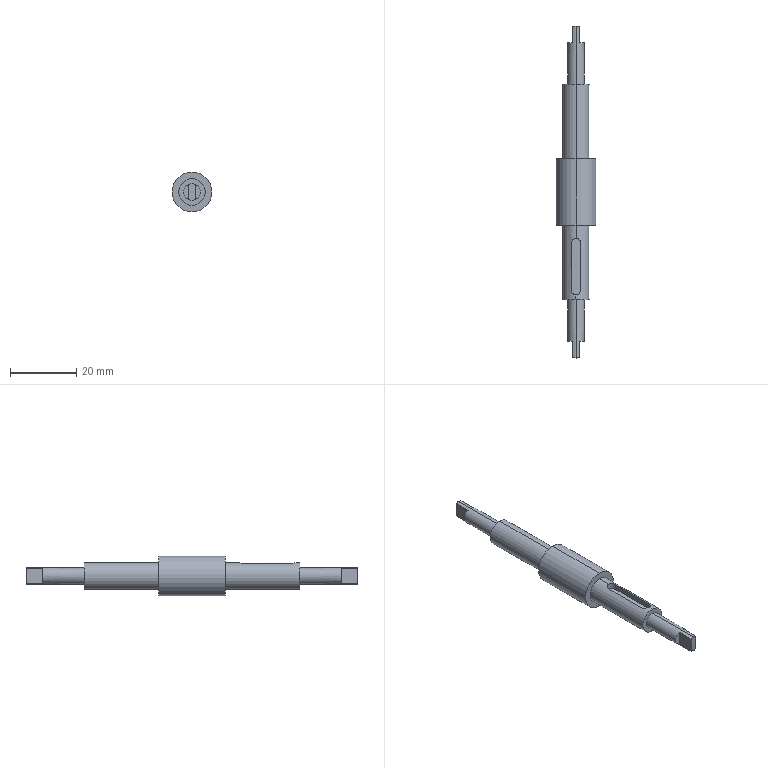Part | SolidWorks | features ICE 7, Extrusion 1 | 1 solid | 29 faces | box 12 x 100 x 12 mm | volume 5018 mm3 | plane 17 | cylinder 12 | commonest cylinder face diameters 5 x4 8 x4 3 x2 12 x2
STEP:
#1=CARTESIAN_POINT('',(0.,-50.,-2.5));
#2=VERTEX_POINT('',#1);
#3=CARTESIAN_POINT('',(1.,-50.,-2.291));
#4=VERTEX_POINT('',#3);
#5=CARTESIAN_POINT('',(0.,-50.,0.));
#6=DIRECTION('',(0.,-1.,0.));
#7=DIRECTION('',(0.,0.,-1.));
#8=AXIS2_PLACEMENT_3D('',#5,#6,#7);
#9=CIRCLE('',#8,2.5);
#10=EDGE_CURVE('',#2,#4,#9,.T.);
#11=ORIENTED_EDGE('',*,*,#10,.F.);
#12=CARTESIAN_POINT('',(0.,-32.5,-2.5));
#13=VERTEX_POINT('',#12);
#14=CARTESIAN_POINT('',(0.,-45.,-2.5));
#15=DIRECTION('',(0.,1.,0.));
#16=VECTOR('',#15,1000.);
#17=LINE('',#14,#16);
#18=EDGE_CURVE('',#2,#13,#17,.T.);
#19=ORIENTED_EDGE('',*,*,#18,.T.);
#20=CARTESIAN_POINT('',(0.,-32.5,2.5));
#21=VERTEX_POINT('',#20);
#22=CARTESIAN_POINT('',(0.,-32.5,0.));
#23=DIRECTION('',(0.,-1.,0.));
#24=DIRECTION('',(0.,0.,-1.));
#25=AXIS2_PLACEMENT_3D('',#22,#23,#24);
#26=CIRCLE('',#25,2.5);
#27=EDGE_CURVE('',#13,#21,#26,.T.);
#28=ORIENTED_EDGE('',*,*,#27,.T.);
#29=CARTESIAN_POINT('',(0.,-50.,2.5));
#30=VERTEX_POINT('',#29);
#31=CARTESIAN_POINT('',(0.,-45.,2.5));
#32=DIRECTION('',(0.,1.,0.));
#33=VECTOR('',#32,1000.);
#34=LINE('',#31,#33);
#35=EDGE_CURVE('',#30,#21,#34,.T.);
#36=ORIENTED_EDGE('',*,*,#35,.F.);
#37=CARTESIAN_POINT('',(1.,-50.,2.291));
#38=VERTEX_POINT('',#37);
#39=CARTESIAN_POINT('',(0.,-50.,0.));
#40=DIRECTION('',(0.,-1.,0.));
#41=DIRECTION('',(0.,0.,-1.));
#42=AXIS2_PLACEMENT_3D('',#39,#40,#41);
#43=CIRCLE('',#42,2.5);
#44=EDGE_CURVE('',#38,#30,#43,.T.);
#45=ORIENTED_EDGE('',*,*,#44,.F.);
#46=CARTESIAN_POINT('',(1.,-45.,2.291));
#47=VERTEX_POINT('',#46);
#48=CARTESIAN_POINT('',(1.,-50.,2.291));
#49=DIRECTION('',(0.,1.,0.));
#50=VECTOR('',#49,1000.);
#51=LINE('',#48,#50);
#52=EDGE_CURVE('',#38,#47,#51,.T.);
#53=ORIENTED_EDGE('',*,*,#52,.T.);
#54=CARTESIAN_POINT('',(1.,-45.,-2.291));
#55=VERTEX_POINT('',#54);
#56=CARTESIAN_POINT('',(0.,-45.,0.));
#57=DIRECTION('',(0.,-1.,0.));
#58=DIRECTION('',(0.,0.,-1.));
#59=AXIS2_PLACEMENT_3D('',#56,#57,#58);
#60=CIRCLE('',#59,2.5);
#61=EDGE_CURVE('',#55,#47,#60,.T.);
#62=ORIENTED_EDGE('',*,*,#61,.F.);
#63=CARTESIAN_POINT('',(1.,-50.,-2.291));
#64=DIRECTION('',(0.,1.,0.));
#65=VECTOR('',#64,1000.);
#66=LINE('',#63,#65);
#67=EDGE_CURVE('',#4,#55,#66,.T.);
#68=ORIENTED_EDGE('',*,*,#67,.F.);
#69=EDGE_LOOP('',(#11,#19,#28,#36,#45,#53,#62,#68));
#70=FACE_OUTER_BOUND('',#69,.T.);
#71=CARTESIAN_POINT('',(0.,-45.,0.));
#72=DIRECTION('',(0.,1.,0.));
#73=DIRECTION('',(0.,0.,1.));
#74=AXIS2_PLACEMENT_3D('',#71,#72,#73);
#75=CYLINDRICAL_SURFACE('',#74,2.5);
#76=ADVANCED_FACE('',(#70),#75,.T.);
#77=CARTESIAN_POINT('',(0.,-32.5,-4.));
#78=VERTEX_POINT('',#77);
#79=CARTESIAN_POINT('',(0.,-32.5,4.));
#80=VERTEX_POINT('',#79);
#81=CARTESIAN_POINT('',(0.,-32.5,0.));
#82=DIRECTION('',(0.,-1.,0.));
#83=DIRECTION('',(0.,0.,-1.));
#84=AXIS2_PLACEMENT_3D('',#81,#82,#83);
#85=CIRCLE('',#84,4.);
#86=EDGE_CURVE('',#78,#80,#85,.T.);
#87=ORIENTED_EDGE('',*,*,#86,.F.);
#88=CARTESIAN_POINT('',(0.,-10.,-4.));
#89=VERTEX_POINT('',#88);
#90=CARTESIAN_POINT('',(0.,-32.5,-4.));
#91=DIRECTION('',(0.,1.,0.));
#92=VECTOR('',#91,1000.);
#93=LINE('',#90,#92);
#94=EDGE_CURVE('',#78,#89,#93,.T.);
#95=ORIENTED_EDGE('',*,*,#94,.T.);
#96=CARTESIAN_POINT('',(0.,-10.,4.));
#97=VERTEX_POINT('',#96);
#98=CARTESIAN_POINT('',(0.,-10.,0.));
#99=DIRECTION('',(0.,-1.,0.));
#100=DIRECTION('',(0.,0.,-1.));
#101=AXIS2_PLACEMENT_3D('',#98,#99,#100);
#102=CIRCLE('',#101,4.);
#103=EDGE_CURVE('',#89,#97,#102,.T.);
#104=ORIENTED_EDGE('',*,*,#103,.T.);
#105=CARTESIAN_POINT('',(0.,-14.,4.));
#106=VERTEX_POINT('',#105);
#107=CARTESIAN_POINT('',(0.,-32.5,4.));
#108=DIRECTION('',(0.,1.,0.));
#109=VECTOR('',#108,1000.);
#110=LINE('',#107,#109);
#111=EDGE_CURVE('',#106,#97,#110,.T.);
#112=ORIENTED_EDGE('',*,*,#111,.F.);
#113=CARTESIAN_POINT('',(1.5,-15.5,3.708));
#114=VERTEX_POINT('',#113);
#115=CARTESIAN_POINT('',(0.,-14.,4.));
#116=CARTESIAN_POINT('',(0.0988,-14.,4.));
#117=CARTESIAN_POINT('',(0.1991,-14.01,3.996));
#118=CARTESIAN_POINT('',(0.3921,-14.049,3.982));
#119=CARTESIAN_POINT('',(0.486,-14.077,3.971));
#120=CARTESIAN_POINT('',(0.6687,-14.154,3.945));
#121=CARTESIAN_POINT('',(0.7547,-14.2,3.929));
#122=CARTESIAN_POINT('',(0.9162,-14.308,3.895));
#123=CARTESIAN_POINT('',(0.9924,-14.371,3.876));
#124=CARTESIAN_POINT('',(1.13,-14.509,3.838));
#125=CARTESIAN_POINT('',(1.191,-14.583,3.819));
#126=CARTESIAN_POINT('',(1.3,-14.745,3.783));
#127=CARTESIAN_POINT('',(1.347,-14.832,3.767));
#128=CARTESIAN_POINT('',(1.459,-15.102,3.725));
#129=CARTESIAN_POINT('',(1.5,-15.3,3.708));
#130=CARTESIAN_POINT('',(1.5,-15.5,3.708));
#131=B_SPLINE_CURVE_WITH_KNOTS('',3,(#115,#116,#117,#118,#119,#120,#121,#122,#123,#124,#125,#126,#127,#128,#129,#130),.UNSPECIFIED.,.F.,.F.,(4,2,2,2,2,2,2,4),(0.002367,0.002663,0.002958,0.003254,0.003549,0.003845,0.00414,0.004731),.UNSPECIFIED.);
#132=EDGE_CURVE('',#106,#114,#131,.T.);
#133=ORIENTED_EDGE('',*,*,#132,.T.);
#134=CARTESIAN_POINT('',(1.5,-29.5,3.708));
#135=VERTEX_POINT('',#134);
#136=CARTESIAN_POINT('',(1.5,-32.5,3.708));
#137=DIRECTION('',(0.,-1.,0.));
#138=VECTOR('',#137,1000.);
#139=LINE('',#136,#138);
#140=EDGE_CURVE('',#114,#135,#139,.T.);
#141=ORIENTED_EDGE('',*,*,#140,.T.);
#142=CARTESIAN_POINT('',(0.,-31.,4.));
#143=VERTEX_POINT('',#142);
#144=CARTESIAN_POINT('',(1.5,-29.5,3.708));
#145=CARTESIAN_POINT('',(1.5,-29.6,3.708));
#146=CARTESIAN_POINT('',(1.49,-29.698,3.712));
#147=CARTESIAN_POINT('',(1.451,-29.891,3.727));
#148=CARTESIAN_POINT('',(1.422,-29.987,3.739));
#149=CARTESIAN_POINT('',(1.309,-30.259,3.781));
#150=CARTESIAN_POINT('',(1.197,-30.424,3.819));
#151=CARTESIAN_POINT('',(0.9232,-30.698,3.895));
#152=CARTESIAN_POINT('',(0.7573,-30.809,3.932));
#153=CARTESIAN_POINT('',(0.4867,-30.922,3.971));
#154=CARTESIAN_POINT('',(0.3912,-30.951,3.982));
#155=CARTESIAN_POINT('',(0.197,-30.99,3.996));
#156=CARTESIAN_POINT('',(0.09895,-31.,4.));
#157=CARTESIAN_POINT('',(0.,-31.,4.));
#158=B_SPLINE_CURVE_WITH_KNOTS('',3,(#144,#145,#146,#147,#148,#149,#150,#151,#152,#153,#154,#155,#156,#157),.UNSPECIFIED.,.F.,.F.,(4,2,2,2,2,2,4),(0.,0.0002959,0.0005918,0.001184,0.001775,0.002071,0.002367),.UNSPECIFIED.);
#159=EDGE_CURVE('',#135,#143,#158,.T.);
#160=ORIENTED_EDGE('',*,*,#159,.T.);
#161=CARTESIAN_POINT('',(0.,-32.5,4.));
#162=DIRECTION('',(0.,1.,0.));
#163=VECTOR('',#162,1000.);
#164=LINE('',#161,#163);
#165=EDGE_CURVE('',#80,#143,#164,.T.);
#166=ORIENTED_EDGE('',*,*,#165,.F.);
#167=EDGE_LOOP('',(#87,#95,#104,#112,#133,#141,#160,#166));
#168=FACE_OUTER_BOUND('',#167,.T.);
#169=CARTESIAN_POINT('',(0.,-32.5,0.));
#170=DIRECTION('',(0.,1.,0.));
#171=DIRECTION('',(0.,0.,1.));
#172=AXIS2_PLACEMENT_3D('',#169,#170,#171);
#173=CYLINDRICAL_SURFACE('',#172,4.);
#174=ADVANCED_FACE('',(#168),#173,.T.);
#175=CARTESIAN_POINT('',(0.,50.,2.5));
#176=VERTEX_POINT('',#175);
#177=CARTESIAN_POINT('',(1.,50.,2.291));
#178=VERTEX_POINT('',#177);
#179=CARTESIAN_POINT('',(0.,50.,0.));
#180=DIRECTION('',(0.,1.,0.));
#181=DIRECTION('',(0.,0.,1.));
#182=AXIS2_PLACEMENT_3D('',#179,#180,#181);
#183=CIRCLE('',#182,2.5);
#184=EDGE_CURVE('',#176,#178,#183,.T.);
#185=ORIENTED_EDGE('',*,*,#184,.F.);
#186=CARTESIAN_POINT('',(0.,32.5,2.5));
#187=VERTEX_POINT('',#186);
#188=CARTESIAN_POINT('',(0.,45.,2.5));
#189=DIRECTION('',(0.,-1.,0.));
#190=VECTOR('',#189,1000.);
#191=LINE('',#188,#190);
#192=EDGE_CURVE('',#176,#187,#191,.T.);
#193=ORIENTED_EDGE('',*,*,#192,.T.);
#194=CARTESIAN_POINT('',(0.,32.5,-2.5));
#195=VERTEX_POINT('',#194);
#196=CARTESIAN_POINT('',(0.,32.5,0.));
#197=DIRECTION('',(0.,1.,0.));
#198=DIRECTION('',(0.,0.,1.));
#199=AXIS2_PLACEMENT_3D('',#196,#197,#198);
#200=CIRCLE('',#199,2.5);
#201=EDGE_CURVE('',#187,#195,#200,.T.);
#202=ORIENTED_EDGE('',*,*,#201,.T.);
#203=CARTESIAN_POINT('',(0.,50.,-2.5));
#204=VERTEX_POINT('',#203);
#205=CARTESIAN_POINT('',(0.,45.,-2.5));
#206=DIRECTION('',(0.,-1.,0.));
#207=VECTOR('',#206,1000.);
#208=LINE('',#205,#207);
#209=EDGE_CURVE('',#204,#195,#208,.T.);
#210=ORIENTED_EDGE('',*,*,#209,.F.);
#211=CARTESIAN_POINT('',(1.,50.,-2.291));
#212=VERTEX_POINT('',#211);
#213=CARTESIAN_POINT('',(0.,50.,0.));
#214=DIRECTION('',(0.,1.,0.));
#215=DIRECTION('',(0.,0.,1.));
#216=AXIS2_PLACEMENT_3D('',#213,#214,#215);
#217=CIRCLE('',#216,2.5);
#218=EDGE_CURVE('',#212,#204,#217,.T.);
#219=ORIENTED_EDGE('',*,*,#218,.F.);
#220=CARTESIAN_POINT('',(1.,45.,-2.291));
#221=VERTEX_POINT('',#220);
#222=CARTESIAN_POINT('',(1.,50.,-2.291));
#223=DIRECTION('',(0.,-1.,0.));
#224=VECTOR('',#223,1000.);
#225=LINE('',#222,#224);
#226=EDGE_CURVE('',#212,#221,#225,.T.);
#227=ORIENTED_EDGE('',*,*,#226,.T.);
#228=CARTESIAN_POINT('',(1.,45.,2.291));
#229=VERTEX_POINT('',#228);
#230=CARTESIAN_POINT('',(0.,45.,0.));
#231=DIRECTION('',(0.,1.,0.));
#232=DIRECTION('',(0.,0.,1.));
#233=AXIS2_PLACEMENT_3D('',#230,#231,#232);
#234=CIRCLE('',#233,2.5);
#235=EDGE_CURVE('',#229,#221,#234,.T.);
#236=ORIENTED_EDGE('',*,*,#235,.F.);
#237=CARTESIAN_POINT('',(1.,50.,2.291));
#238=DIRECTION('',(0.,-1.,0.));
#239=VECTOR('',#238,1000.);
#240=LINE('',#237,#239);
#241=EDGE_CURVE('',#178,#229,#240,.T.);
#242=ORIENTED_EDGE('',*,*,#241,.F.);
#243=EDGE_LOOP('',(#185,#193,#202,#210,#219,#227,#236,#242));
#244=FACE_OUTER_BOUND('',#243,.T.);
#245=CARTESIAN_POINT('',(0.,45.,0.));
#246=DIRECTION('',(0.,-1.,0.));
#247=DIRECTION('',(0.,0.,-1.));
#248=AXIS2_PLACEMENT_3D('',#245,#246,#247);
#249=CYLINDRICAL_SURFACE('',#248,2.5);
#250=ADVANCED_FACE('',(#244),#249,.T.);
#251=CARTESIAN_POINT('',(0.,32.5,4.));
#252=VERTEX_POINT('',#251);
#253=CARTESIAN_POINT('',(0.,32.5,-4.));
#254=VERTEX_POINT('',#253);
#255=CARTESIAN_POINT('',(0.,32.5,0.));
#256=DIRECTION('',(0.,1.,0.));
#257=DIRECTION('',(0.,0.,1.));
#258=AXIS2_PLACEMENT_3D('',#255,#256,#257);
#259=CIRCLE('',#258,4.);
#260=EDGE_CURVE('',#252,#254,#259,.T.);
#261=ORIENTED_EDGE('',*,*,#260,.F.);
#262=CARTESIAN_POINT('',(0.,10.,4.));
#263=VERTEX_POINT('',#262);
#264=CARTESIAN_POINT('',(0.,32.5,4.));
#265=DIRECTION('',(0.,-1.,0.));
#266=VECTOR('',#265,1000.);
#267=LINE('',#264,#266);
#268=EDGE_CURVE('',#252,#263,#267,.T.);
#269=ORIENTED_EDGE('',*,*,#268,.T.);
#270=CARTESIAN_POINT('',(0.,10.,-4.));
#271=VERTEX_POINT('',#270);
#272=CARTESIAN_POINT('',(0.,10.,0.));
#273=DIRECTION('',(0.,1.,0.));
#274=DIRECTION('',(0.,0.,1.));
#275=AXIS2_PLACEMENT_3D('',#272,#273,#274);
#276=CIRCLE('',#275,4.);
#277=EDGE_CURVE('',#263,#271,#276,.T.);
#278=ORIENTED_EDGE('',*,*,#277,.T.);
#279=CARTESIAN_POINT('',(0.,32.5,-4.));
#280=DIRECTION('',(0.,-1.,0.));
#281=VECTOR('',#280,1000.);
#282=LINE('',#279,#281);
#283=EDGE_CURVE('',#254,#271,#282,.T.);
#284=ORIENTED_EDGE('',*,*,#283,.F.);
#285=EDGE_LOOP('',(#261,#269,#278,#284));
#286=FACE_OUTER_BOUND('',#285,.T.);
#287=CARTESIAN_POINT('',(0.,32.5,0.));
#288=DIRECTION('',(0.,-1.,0.));
#289=DIRECTION('',(0.,0.,-1.));
#290=AXIS2_PLACEMENT_3D('',#287,#288,#289);
#291=CYLINDRICAL_SURFACE('',#290,4.);
#292=ADVANCED_FACE('',(#286),#291,.T.);
#293=CARTESIAN_POINT('',(0.,10.,6.));
#294=VERTEX_POINT('',#293);
#295=CARTESIAN_POINT('',(0.,10.,-6.));
#296=VERTEX_POINT('',#295);
#297=CARTESIAN_POINT('',(0.,10.,0.));
#298=DIRECTION('',(0.,1.,0.));
#299=DIRECTION('',(0.,0.,1.));
#300=AXIS2_PLACEMENT_3D('',#297,#298,#299);
#301=CIRCLE('',#300,6.);
#302=EDGE_CURVE('',#294,#296,#301,.T.);
#303=ORIENTED_EDGE('',*,*,#302,.F.);
#304=CARTESIAN_POINT('',(0.,-10.,6.));
#305=VERTEX_POINT('',#304);
#306=CARTESIAN_POINT('',(0.,10.,6.));
#307=DIRECTION('',(0.,-1.,0.));
#308=VECTOR('',#307,1000.);
#309=LINE('',#306,#308);
#310=EDGE_CURVE('',#294,#305,#309,.T.);
#311=ORIENTED_EDGE('',*,*,#310,.T.);
#312=CARTESIAN_POINT('',(0.,-10.,-6.));
#313=VERTEX_POINT('',#312);
#314=CARTESIAN_POINT('',(0.,-10.,0.));
#315=DIRECTION('',(0.,1.,0.));
#316=DIRECTION('',(0.,0.,1.));
#317=AXIS2_PLACEMENT_3D('',#314,#315,#316);
#318=CIRCLE('',#317,6.);
#319=EDGE_CURVE('',#305,#313,#318,.T.);
#320=ORIENTED_EDGE('',*,*,#319,.T.);
#321=CARTESIAN_POINT('',(0.,10.,-6.));
#322=DIRECTION('',(0.,-1.,0.));
#323=VECTOR('',#322,1000.);
#324=LINE('',#321,#323);
#325=EDGE_CURVE('',#296,#313,#324,.T.);
#326=ORIENTED_EDGE('',*,*,#325,.F.);
#327=EDGE_LOOP('',(#303,#311,#320,#326));
#328=FACE_OUTER_BOUND('',#327,.T.);
#329=CARTESIAN_POINT('',(0.,10.,0.));
#330=DIRECTION('',(0.,-1.,0.));
#331=DIRECTION('',(0.,0.,-1.));
#332=AXIS2_PLACEMENT_3D('',#329,#330,#331);
#333=CYLINDRICAL_SURFACE('',#332,6.);
#334=ADVANCED_FACE('',(#328),#333,.T.);
#335=CARTESIAN_POINT('',(1.,45.,-2.291));
#336=DIRECTION('',(0.,0.,-1.));
#337=VECTOR('',#336,1000.);
#338=LINE('',#335,#337);
#339=EDGE_CURVE('',#229,#221,#338,.T.);
#340=ORIENTED_EDGE('',*,*,#339,.F.);
#341=ORIENTED_EDGE('',*,*,#235,.T.);
#342=EDGE_LOOP('',(#340,#341));
#343=FACE_OUTER_BOUND('',#342,.T.);
#344=CARTESIAN_POINT('',(0.,45.,0.));
#345=DIRECTION('',(0.,1.,0.));
#346=DIRECTION('',(0.,0.,1.));
#347=AXIS2_PLACEMENT_3D('',#344,#345,#346);
#348=PLANE('',#347);
#349=ADVANCED_FACE('',(#343),#348,.T.);
#350=CARTESIAN_POINT('',(1.,-45.,2.291));
#351=DIRECTION('',(0.,0.,1.));
#352=VECTOR('',#351,1000.);
#353=LINE('',#350,#352);
#354=EDGE_CURVE('',#55,#47,#353,.T.);
#355=ORIENTED_EDGE('',*,*,#354,.F.);
#356=ORIENTED_EDGE('',*,*,#61,.T.);
#357=EDGE_LOOP('',(#355,#356));
#358=FACE_OUTER_BOUND('',#357,.T.);
#359=CARTESIAN_POINT('',(0.,-45.,0.));
#360=DIRECTION('',(0.,-1.,0.));
#361=DIRECTION('',(0.,0.,-1.));
#362=AXIS2_PLACEMENT_3D('',#359,#360,#361);
#363=PLANE('',#362);
#364=ADVANCED_FACE('',(#358),#363,.T.);
#365=ORIENTED_EDGE('',*,*,#310,.F.);
#366=CARTESIAN_POINT('',(0.,10.,0.));
#367=DIRECTION('',(0.,1.,0.));
#368=DIRECTION('',(0.,0.,1.));
#369=AXIS2_PLACEMENT_3D('',#366,#367,#368);
#370=CIRCLE('',#369,6.);
#371=EDGE_CURVE('',#296,#294,#370,.T.);
#372=ORIENTED_EDGE('',*,*,#371,.F.);
#373=ORIENTED_EDGE('',*,*,#325,.T.);
#374=CARTESIAN_POINT('',(0.,-10.,0.));
#375=DIRECTION('',(0.,1.,0.));
#376=DIRECTION('',(0.,0.,1.));
#377=AXIS2_PLACEMENT_3D('',#374,#375,#376);
#378=CIRCLE('',#377,6.);
#379=EDGE_CURVE('',#313,#305,#378,.T.);
#380=ORIENTED_EDGE('',*,*,#379,.T.);
#381=EDGE_LOOP('',(#365,#372,#373,#380));
#382=FACE_OUTER_BOUND('',#381,.T.);
#383=CARTESIAN_POINT('',(0.,10.,0.));
#384=DIRECTION('',(0.,-1.,0.));
#385=DIRECTION('',(0.,0.,-1.));
#386=AXIS2_PLACEMENT_3D('',#383,#384,#385);
#387=CYLINDRICAL_SURFACE('',#386,6.);
#388=ADVANCED_FACE('',(#382),#387,.T.);
#389=CARTESIAN_POINT('',(0.,10.,0.));
#390=DIRECTION('',(0.,1.,0.));
#391=DIRECTION('',(0.,0.,1.));
#392=AXIS2_PLACEMENT_3D('',#389,#390,#391);
#393=CIRCLE('',#392,4.);
#394=EDGE_CURVE('',#271,#263,#393,.T.);
#395=ORIENTED_EDGE('',*,*,#394,.F.);
#396=ORIENTED_EDGE('',*,*,#277,.F.);
#397=EDGE_LOOP('',(#395,#396));
#398=FACE_BOUND('',#397,.T.);
#399=ORIENTED_EDGE('',*,*,#371,.T.);
#400=ORIENTED_EDGE('',*,*,#302,.T.);
#401=EDGE_LOOP('',(#399,#400));
#402=FACE_OUTER_BOUND('',#401,.T.);
#403=CARTESIAN_POINT('',(0.,10.,0.));
#404=DIRECTION('',(0.,1.,0.));
#405=DIRECTION('',(0.,0.,1.));
#406=AXIS2_PLACEMENT_3D('',#403,#404,#405);
#407=PLANE('',#406);
#408=ADVANCED_FACE('',(#398,#402),#407,.T.);
#409=CARTESIAN_POINT('',(0.,-10.,0.));
#410=DIRECTION('',(0.,-1.,0.));
#411=DIRECTION('',(0.,0.,-1.));
#412=AXIS2_PLACEMENT_3D('',#409,#410,#411);
#413=CIRCLE('',#412,4.);
#414=EDGE_CURVE('',#97,#89,#413,.T.);
#415=ORIENTED_EDGE('',*,*,#414,.F.);
#416=ORIENTED_EDGE('',*,*,#103,.F.);
#417=EDGE_LOOP('',(#415,#416));
#418=FACE_BOUND('',#417,.T.);
#419=ORIENTED_EDGE('',*,*,#379,.F.);
#420=ORIENTED_EDGE('',*,*,#319,.F.);
#421=EDGE_LOOP('',(#419,#420));
#422=FACE_OUTER_BOUND('',#421,.T.);
#423=CARTESIAN_POINT('',(0.,-10.,0.));
#424=DIRECTION('',(0.,1.,0.));
#425=DIRECTION('',(0.,0.,1.));
#426=AXIS2_PLACEMENT_3D('',#423,#424,#425);
#427=PLANE('',#426);
#428=ADVANCED_FACE('',(#418,#422),#427,.F.);
#429=ORIENTED_EDGE('',*,*,#268,.F.);
#430=CARTESIAN_POINT('',(0.,32.5,0.));
#431=DIRECTION('',(0.,1.,0.));
#432=DIRECTION('',(0.,0.,1.));
#433=AXIS2_PLACEMENT_3D('',#430,#431,#432);
#434=CIRCLE('',#433,4.);
#435=EDGE_CURVE('',#254,#252,#434,.T.);
#436=ORIENTED_EDGE('',*,*,#435,.F.);
#437=ORIENTED_EDGE('',*,*,#283,.T.);
#438=ORIENTED_EDGE('',*,*,#394,.T.);
#439=EDGE_LOOP('',(#429,#436,#437,#438));
#440=FACE_OUTER_BOUND('',#439,.T.);
#441=CARTESIAN_POINT('',(0.,32.5,0.));
#442=DIRECTION('',(0.,-1.,0.));
#443=DIRECTION('',(0.,0.,-1.));
#444=AXIS2_PLACEMENT_3D('',#441,#442,#443);
#445=CYLINDRICAL_SURFACE('',#444,4.);
#446=ADVANCED_FACE('',(#440),#445,.T.);
#447=CARTESIAN_POINT('',(0.,32.5,0.));
#448=DIRECTION('',(0.,1.,0.));
#449=DIRECTION('',(0.,0.,1.));
#450=AXIS2_PLACEMENT_3D('',#447,#448,#449);
#451=CIRCLE('',#450,2.5);
#452=EDGE_CURVE('',#195,#187,#451,.T.);
#453=ORIENTED_EDGE('',*,*,#452,.F.);
#454=ORIENTED_EDGE('',*,*,#201,.F.);
#455=EDGE_LOOP('',(#453,#454));
#456=FACE_BOUND('',#455,.T.);
#457=ORIENTED_EDGE('',*,*,#435,.T.);
#458=ORIENTED_EDGE('',*,*,#260,.T.);
#459=EDGE_LOOP('',(#457,#458));
#460=FACE_OUTER_BOUND('',#459,.T.);
#461=CARTESIAN_POINT('',(0.,32.5,0.));
#462=DIRECTION('',(0.,1.,0.));
#463=DIRECTION('',(0.,0.,1.));
#464=AXIS2_PLACEMENT_3D('',#461,#462,#463);
#465=PLANE('',#464);
#466=ADVANCED_FACE('',(#456,#460),#465,.T.);
#467=ORIENTED_EDGE('',*,*,#192,.F.);
#468=CARTESIAN_POINT('',(-1.,50.,2.291));
#469=VERTEX_POINT('',#468);
#470=CARTESIAN_POINT('',(0.,50.,0.));
#471=DIRECTION('',(0.,1.,0.));
#472=DIRECTION('',(0.,0.,1.));
#473=AXIS2_PLACEMENT_3D('',#470,#471,#472);
#474=CIRCLE('',#473,2.5);
#475=EDGE_CURVE('',#469,#176,#474,.T.);
#476=ORIENTED_EDGE('',*,*,#475,.F.);
#477=CARTESIAN_POINT('',(-1.,45.,2.291));
#478=VERTEX_POINT('',#477);
#479=CARTESIAN_POINT('',(-1.,50.,2.291));
#480=DIRECTION('',(0.,-1.,0.));
#481=VECTOR('',#480,1000.);
#482=LINE('',#479,#481);
#483=EDGE_CURVE('',#469,#478,#482,.T.);
#484=ORIENTED_EDGE('',*,*,#483,.T.);
#485=CARTESIAN_POINT('',(-1.,45.,-2.291));
#486=VERTEX_POINT('',#485);
#487=CARTESIAN_POINT('',(0.,45.,0.));
#488=DIRECTION('',(0.,1.,0.));
#489=DIRECTION('',(0.,0.,1.));
#490=AXIS2_PLACEMENT_3D('',#487,#488,#489);
#491=CIRCLE('',#490,2.5);
#492=EDGE_CURVE('',#486,#478,#491,.T.);
#493=ORIENTED_EDGE('',*,*,#492,.F.);
#494=CARTESIAN_POINT('',(-1.,50.,-2.291));
#495=VERTEX_POINT('',#494);
#496=CARTESIAN_POINT('',(-1.,50.,-2.291));
#497=DIRECTION('',(0.,-1.,0.));
#498=VECTOR('',#497,1000.);
#499=LINE('',#496,#498);
#500=EDGE_CURVE('',#495,#486,#499,.T.);
#501=ORIENTED_EDGE('',*,*,#500,.F.);
#502=CARTESIAN_POINT('',(0.,50.,0.));
#503=DIRECTION('',(0.,1.,0.));
#504=DIRECTION('',(0.,0.,1.));
#505=AXIS2_PLACEMENT_3D('',#502,#503,#504);
#506=CIRCLE('',#505,2.5);
#507=EDGE_CURVE('',#204,#495,#506,.T.);
#508=ORIENTED_EDGE('',*,*,#507,.F.);
#509=ORIENTED_EDGE('',*,*,#209,.T.);
#510=ORIENTED_EDGE('',*,*,#452,.T.);
#511=EDGE_LOOP('',(#467,#476,#484,#493,#501,#508,#509,#510));
#512=FACE_OUTER_BOUND('',#511,.T.);
#513=CARTESIAN_POINT('',(0.,45.,0.));
#514=DIRECTION('',(0.,-1.,0.));
#515=DIRECTION('',(0.,0.,-1.));
#516=AXIS2_PLACEMENT_3D('',#513,#514,#515);
#517=CYLINDRICAL_SURFACE('',#516,2.5);
#518=ADVANCED_FACE('',(#512),#517,.T.);
#519=CARTESIAN_POINT('',(-1.,45.,-2.291));
#520=DIRECTION('',(0.,0.,1.));
#521=VECTOR('',#520,1000.);
#522=LINE('',#519,#521);
#523=EDGE_CURVE('',#486,#478,#522,.T.);
#524=ORIENTED_EDGE('',*,*,#523,.F.);
#525=ORIENTED_EDGE('',*,*,#492,.T.);
#526=EDGE_LOOP('',(#524,#525));
#527=FACE_OUTER_BOUND('',#526,.T.);
#528=CARTESIAN_POINT('',(0.,45.,0.));
#529=DIRECTION('',(0.,1.,0.));
#530=DIRECTION('',(0.,0.,1.));
#531=AXIS2_PLACEMENT_3D('',#528,#529,#530);
#532=PLANE('',#531);
#533=ADVANCED_FACE('',(#527),#532,.T.);
#534=ORIENTED_EDGE('',*,*,#94,.F.);
#535=CARTESIAN_POINT('',(0.,-32.5,0.));
#536=DIRECTION('',(0.,-1.,0.));
#537=DIRECTION('',(0.,0.,-1.));
#538=AXIS2_PLACEMENT_3D('',#535,#536,#537);
#539=CIRCLE('',#538,4.);
#540=EDGE_CURVE('',#80,#78,#539,.T.);
#541=ORIENTED_EDGE('',*,*,#540,.F.);
#542=ORIENTED_EDGE('',*,*,#165,.T.);
#543=CARTESIAN_POINT('',(-1.5,-29.5,3.708));
#544=VERTEX_POINT('',#543);
#545=CARTESIAN_POINT('',(0.,-31.,4.));
#546=CARTESIAN_POINT('',(-0.0988,-31.,4.));
#547=CARTESIAN_POINT('',(-0.1991,-30.99,3.996));
#548=CARTESIAN_POINT('',(-0.3921,-30.951,3.982));
#549=CARTESIAN_POINT('',(-0.486,-30.923,3.971));
#550=CARTESIAN_POINT('',(-0.6687,-30.846,3.945));
#551=CARTESIAN_POINT('',(-0.7547,-30.8,3.929));
#552=CARTESIAN_POINT('',(-0.9162,-30.692,3.895));
#553=CARTESIAN_POINT('',(-0.9924,-30.629,3.876));
#554=CARTESIAN_POINT('',(-1.13,-30.491,3.838));
#555=CARTESIAN_POINT('',(-1.191,-30.417,3.819));
#556=CARTESIAN_POINT('',(-1.3,-30.255,3.783));
#557=CARTESIAN_POINT('',(-1.347,-30.168,3.767));
#558=CARTESIAN_POINT('',(-1.459,-29.898,3.725));
#559=CARTESIAN_POINT('',(-1.5,-29.7,3.708));
#560=CARTESIAN_POINT('',(-1.5,-29.5,3.708));
#561=B_SPLINE_CURVE_WITH_KNOTS('',3,(#545,#546,#547,#548,#549,#550,#551,#552,#553,#554,#555,#556,#557,#558,#559,#560),.UNSPECIFIED.,.F.,.F.,(4,2,2,2,2,2,2,4),(0.002367,0.002663,0.002958,0.003254,0.003549,0.003845,0.00414,0.004731),.UNSPECIFIED.);
#562=EDGE_CURVE('',#143,#544,#561,.T.);
#563=ORIENTED_EDGE('',*,*,#562,.T.);
#564=CARTESIAN_POINT('',(-1.5,-15.5,3.708));
#565=VERTEX_POINT('',#564);
#566=CARTESIAN_POINT('',(-1.5,-32.5,3.708));
#567=DIRECTION('',(0.,1.,0.));
#568=VECTOR('',#567,1000.);
#569=LINE('',#566,#568);
#570=EDGE_CURVE('',#544,#565,#569,.T.);
#571=ORIENTED_EDGE('',*,*,#570,.T.);
#572=CARTESIAN_POINT('',(-1.5,-15.5,3.708));
#573=CARTESIAN_POINT('',(-1.5,-15.4,3.708));
#574=CARTESIAN_POINT('',(-1.49,-15.302,3.712));
#575=CARTESIAN_POINT('',(-1.451,-15.109,3.727));
#576=CARTESIAN_POINT('',(-1.422,-15.013,3.739));
#577=CARTESIAN_POINT('',(-1.309,-14.741,3.781));
#578=CARTESIAN_POINT('',(-1.197,-14.576,3.819));
#579=CARTESIAN_POINT('',(-0.9232,-14.302,3.895));
#580=CARTESIAN_POINT('',(-0.7573,-14.191,3.932));
#581=CARTESIAN_POINT('',(-0.4867,-14.078,3.971));
#582=CARTESIAN_POINT('',(-0.3912,-14.049,3.982));
#583=CARTESIAN_POINT('',(-0.197,-14.01,3.996));
#584=CARTESIAN_POINT('',(-0.09895,-14.,4.));
#585=CARTESIAN_POINT('',(0.,-14.,4.));
#586=B_SPLINE_CURVE_WITH_KNOTS('',3,(#572,#573,#574,#575,#576,#577,#578,#579,#580,#581,#582,#583,#584,#585),.UNSPECIFIED.,.F.,.F.,(4,2,2,2,2,2,4),(0.,0.0002959,0.0005918,0.001184,0.001775,0.002071,0.002367),.UNSPECIFIED.);
#587=EDGE_CURVE('',#565,#106,#586,.T.);
#588=ORIENTED_EDGE('',*,*,#587,.T.);
#589=ORIENTED_EDGE('',*,*,#111,.T.);
#590=ORIENTED_EDGE('',*,*,#414,.T.);
#591=EDGE_LOOP('',(#534,#541,#542,#563,#571,#588,#589,#590));
#592=FACE_OUTER_BOUND('',#591,.T.);
#593=CARTESIAN_POINT('',(0.,-32.5,0.));
#594=DIRECTION('',(0.,1.,0.));
#595=DIRECTION('',(0.,0.,1.));
#596=AXIS2_PLACEMENT_3D('',#593,#594,#595);
#597=CYLINDRICAL_SURFACE('',#596,4.);
#598=ADVANCED_FACE('',(#592),#597,.T.);
#599=CARTESIAN_POINT('',(0.,-32.5,0.));
#600=DIRECTION('',(0.,-1.,0.));
#601=DIRECTION('',(0.,0.,-1.));
#602=AXIS2_PLACEMENT_3D('',#599,#600,#601);
#603=CIRCLE('',#602,2.5);
#604=EDGE_CURVE('',#21,#13,#603,.T.);
#605=ORIENTED_EDGE('',*,*,#604,.F.);
#606=ORIENTED_EDGE('',*,*,#27,.F.);
#607=EDGE_LOOP('',(#605,#606));
#608=FACE_BOUND('',#607,.T.);
#609=ORIENTED_EDGE('',*,*,#540,.T.);
#610=ORIENTED_EDGE('',*,*,#86,.T.);
#611=EDGE_LOOP('',(#609,#610));
#612=FACE_OUTER_BOUND('',#611,.T.);
#613=CARTESIAN_POINT('',(0.,-32.5,0.));
#614=DIRECTION('',(0.,-1.,0.));
#615=DIRECTION('',(0.,0.,-1.));
#616=AXIS2_PLACEMENT_3D('',#613,#614,#615);
#617=PLANE('',#616);
#618=ADVANCED_FACE('',(#608,#612),#617,.T.);
#619=ORIENTED_EDGE('',*,*,#18,.F.);
#620=CARTESIAN_POINT('',(-1.,-50.,-2.291));
#621=VERTEX_POINT('',#620);
#622=CARTESIAN_POINT('',(0.,-50.,0.));
#623=DIRECTION('',(0.,-1.,0.));
#624=DIRECTION('',(0.,0.,-1.));
#625=AXIS2_PLACEMENT_3D('',#622,#623,#624);
#626=CIRCLE('',#625,2.5);
#627=EDGE_CURVE('',#621,#2,#626,.T.);
#628=ORIENTED_EDGE('',*,*,#627,.F.);
#629=CARTESIAN_POINT('',(-1.,-45.,-2.291));
#630=VERTEX_POINT('',#629);
#631=CARTESIAN_POINT('',(-1.,-50.,-2.291));
#632=DIRECTION('',(0.,1.,0.));
#633=VECTOR('',#632,1000.);
#634=LINE('',#631,#633);
#635=EDGE_CURVE('',#621,#630,#634,.T.);
#636=ORIENTED_EDGE('',*,*,#635,.T.);
#637=CARTESIAN_POINT('',(-1.,-45.,2.291));
#638=VERTEX_POINT('',#637);
#639=CARTESIAN_POINT('',(0.,-45.,0.));
#640=DIRECTION('',(0.,-1.,0.));
#641=DIRECTION('',(0.,0.,-1.));
#642=AXIS2_PLACEMENT_3D('',#639,#640,#641);
#643=CIRCLE('',#642,2.5);
#644=EDGE_CURVE('',#638,#630,#643,.T.);
#645=ORIENTED_EDGE('',*,*,#644,.F.);
#646=CARTESIAN_POINT('',(-1.,-50.,2.291));
#647=VERTEX_POINT('',#646);
#648=CARTESIAN_POINT('',(-1.,-50.,2.291));
#649=DIRECTION('',(0.,1.,0.));
#650=VECTOR('',#649,1000.);
#651=LINE('',#648,#650);
#652=EDGE_CURVE('',#647,#638,#651,.T.);
#653=ORIENTED_EDGE('',*,*,#652,.F.);
#654=CARTESIAN_POINT('',(0.,-50.,0.));
#655=DIRECTION('',(0.,-1.,0.));
#656=DIRECTION('',(0.,0.,-1.));
#657=AXIS2_PLACEMENT_3D('',#654,#655,#656);
#658=CIRCLE('',#657,2.5);
#659=EDGE_CURVE('',#30,#647,#658,.T.);
#660=ORIENTED_EDGE('',*,*,#659,.F.);
#661=ORIENTED_EDGE('',*,*,#35,.T.);
#662=ORIENTED_EDGE('',*,*,#604,.T.);
#663=EDGE_LOOP('',(#619,#628,#636,#645,#653,#660,#661,#662));
#664=FACE_OUTER_BOUND('',#663,.T.);
#665=CARTESIAN_POINT('',(0.,-45.,0.));
#666=DIRECTION('',(0.,1.,0.));
#667=DIRECTION('',(0.,0.,1.));
#668=AXIS2_PLACEMENT_3D('',#665,#666,#667);
#669=CYLINDRICAL_SURFACE('',#668,2.5);
#670=ADVANCED_FACE('',(#664),#669,.T.);
#671=CARTESIAN_POINT('',(-1.,-45.,2.291));
#672=DIRECTION('',(0.,0.,-1.));
#673=VECTOR('',#672,1000.);
#674=LINE('',#671,#673);
#675=EDGE_CURVE('',#638,#630,#674,.T.);
#676=ORIENTED_EDGE('',*,*,#675,.F.);
#677=ORIENTED_EDGE('',*,*,#644,.T.);
#678=EDGE_LOOP('',(#676,#677));
#679=FACE_OUTER_BOUND('',#678,.T.);
#680=CARTESIAN_POINT('',(0.,-45.,0.));
#681=DIRECTION('',(0.,-1.,0.));
#682=DIRECTION('',(0.,0.,-1.));
#683=AXIS2_PLACEMENT_3D('',#680,#681,#682);
#684=PLANE('',#683);
#685=ADVANCED_FACE('',(#679),#684,.T.);
#686=ORIENTED_EDGE('',*,*,#675,.T.);
#687=ORIENTED_EDGE('',*,*,#635,.F.);
#688=CARTESIAN_POINT('',(-1.,-50.,2.291));
#689=DIRECTION('',(0.,0.,-1.));
#690=VECTOR('',#689,1000.);
#691=LINE('',#688,#690);
#692=EDGE_CURVE('',#647,#621,#691,.T.);
#693=ORIENTED_EDGE('',*,*,#692,.F.);
#694=ORIENTED_EDGE('',*,*,#652,.T.);
#695=EDGE_LOOP('',(#686,#687,#693,#694));
#696=FACE_OUTER_BOUND('',#695,.T.);
#697=CARTESIAN_POINT('',(-1.,-50.,2.291));
#698=DIRECTION('',(1.,0.,0.));
#699=DIRECTION('',(0.,0.,-1.));
#700=AXIS2_PLACEMENT_3D('',#697,#698,#699);
#701=PLANE('',#700);
#702=ADVANCED_FACE('',(#696),#701,.F.);
#703=ORIENTED_EDGE('',*,*,#354,.T.);
#704=ORIENTED_EDGE('',*,*,#52,.F.);
#705=CARTESIAN_POINT('',(1.,-50.,2.291));
#706=DIRECTION('',(0.,0.,1.));
#707=VECTOR('',#706,1000.);
#708=LINE('',#705,#707);
#709=EDGE_CURVE('',#4,#38,#708,.T.);
#710=ORIENTED_EDGE('',*,*,#709,.F.);
#711=ORIENTED_EDGE('',*,*,#67,.T.);
#712=EDGE_LOOP('',(#703,#704,#710,#711));
#713=FACE_OUTER_BOUND('',#712,.T.);
#714=CARTESIAN_POINT('',(1.,-50.,2.291));
#715=DIRECTION('',(-1.,0.,0.));
#716=DIRECTION('',(0.,0.,1.));
#717=AXIS2_PLACEMENT_3D('',#714,#715,#716);
#718=PLANE('',#717);
#719=ADVANCED_FACE('',(#713),#718,.F.);
#720=ORIENTED_EDGE('',*,*,#44,.T.);
#721=ORIENTED_EDGE('',*,*,#659,.T.);
#722=ORIENTED_EDGE('',*,*,#692,.T.);
#723=ORIENTED_EDGE('',*,*,#627,.T.);
#724=ORIENTED_EDGE('',*,*,#10,.T.);
#725=ORIENTED_EDGE('',*,*,#709,.T.);
#726=EDGE_LOOP('',(#720,#721,#722,#723,#724,#725));
#727=FACE_OUTER_BOUND('',#726,.T.);
#728=CARTESIAN_POINT('',(0.,-50.,0.));
#729=DIRECTION('',(0.,-1.,0.));
#730=DIRECTION('',(0.,0.,-1.));
#731=AXIS2_PLACEMENT_3D('',#728,#729,#730);
#732=PLANE('',#731);
#733=ADVANCED_FACE('',(#727),#732,.T.);
#734=ORIENTED_EDGE('',*,*,#523,.T.);
#735=ORIENTED_EDGE('',*,*,#483,.F.);
#736=CARTESIAN_POINT('',(-1.,50.,-2.291));
#737=DIRECTION('',(0.,0.,1.));
#738=VECTOR('',#737,1000.);
#739=LINE('',#736,#738);
#740=EDGE_CURVE('',#495,#469,#739,.T.);
#741=ORIENTED_EDGE('',*,*,#740,.F.);
#742=ORIENTED_EDGE('',*,*,#500,.T.);
#743=EDGE_LOOP('',(#734,#735,#741,#742));
#744=FACE_OUTER_BOUND('',#743,.T.);
#745=CARTESIAN_POINT('',(-1.,50.,-2.291));
#746=DIRECTION('',(1.,0.,0.));
#747=DIRECTION('',(0.,0.,-1.));
#748=AXIS2_PLACEMENT_3D('',#745,#746,#747);
#749=PLANE('',#748);
#750=ADVANCED_FACE('',(#744),#749,.F.);
#751=ORIENTED_EDGE('',*,*,#339,.T.);
#752=ORIENTED_EDGE('',*,*,#226,.F.);
#753=CARTESIAN_POINT('',(1.,50.,-2.291));
#754=DIRECTION('',(0.,0.,-1.));
#755=VECTOR('',#754,1000.);
#756=LINE('',#753,#755);
#757=EDGE_CURVE('',#178,#212,#756,.T.);
#758=ORIENTED_EDGE('',*,*,#757,.F.);
#759=ORIENTED_EDGE('',*,*,#241,.T.);
#760=EDGE_LOOP('',(#751,#752,#758,#759));
#761=FACE_OUTER_BOUND('',#760,.T.);
#762=CARTESIAN_POINT('',(1.,50.,-2.291));
#763=DIRECTION('',(-1.,0.,0.));
#764=DIRECTION('',(0.,0.,1.));
#765=AXIS2_PLACEMENT_3D('',#762,#763,#764);
#766=PLANE('',#765);
#767=ADVANCED_FACE('',(#761),#766,.F.);
#768=ORIENTED_EDGE('',*,*,#218,.T.);
#769=ORIENTED_EDGE('',*,*,#507,.T.);
#770=ORIENTED_EDGE('',*,*,#740,.T.);
#771=ORIENTED_EDGE('',*,*,#475,.T.);
#772=ORIENTED_EDGE('',*,*,#184,.T.);
#773=ORIENTED_EDGE('',*,*,#757,.T.);
#774=EDGE_LOOP('',(#768,#769,#770,#771,#772,#773));
#775=FACE_OUTER_BOUND('',#774,.T.);
#776=CARTESIAN_POINT('',(0.,50.,0.));
#777=DIRECTION('',(0.,1.,0.));
#778=DIRECTION('',(0.,0.,1.));
#779=AXIS2_PLACEMENT_3D('',#776,#777,#778);
#780=PLANE('',#779);
#781=ADVANCED_FACE('',(#775),#780,.T.);
#782=CARTESIAN_POINT('',(1.5,-29.5,2.));
#783=VERTEX_POINT('',#782);
#784=CARTESIAN_POINT('',(1.5,-29.5,2.));
#785=DIRECTION('',(0.,0.,1.));
#786=VECTOR('',#785,1000.);
#787=LINE('',#784,#786);
#788=EDGE_CURVE('',#783,#135,#787,.T.);
#789=ORIENTED_EDGE('',*,*,#788,.F.);
#790=CARTESIAN_POINT('',(-1.5,-29.5,2.));
#791=VERTEX_POINT('',#790);
#792=CARTESIAN_POINT('',(0.,-29.5,2.));
#793=DIRECTION('',(0.,0.,1.));
#794=DIRECTION('',(1.,0.,0.));
#795=AXIS2_PLACEMENT_3D('',#792,#793,#794);
#796=CIRCLE('',#795,1.5);
#797=EDGE_CURVE('',#791,#783,#796,.T.);
#798=ORIENTED_EDGE('',*,*,#797,.F.);
#799=CARTESIAN_POINT('',(-1.5,-29.5,2.));
#800=DIRECTION('',(0.,0.,1.));
#801=VECTOR('',#800,1000.);
#802=LINE('',#799,#801);
#803=EDGE_CURVE('',#791,#544,#802,.T.);
#804=ORIENTED_EDGE('',*,*,#803,.T.);
#805=ORIENTED_EDGE('',*,*,#562,.F.);
#806=ORIENTED_EDGE('',*,*,#159,.F.);
#807=EDGE_LOOP('',(#789,#798,#804,#805,#806));
#808=FACE_OUTER_BOUND('',#807,.T.);
#809=CARTESIAN_POINT('',(0.,-29.5,2.));
#810=DIRECTION('',(0.,0.,1.));
#811=DIRECTION('',(1.,0.,0.));
#812=AXIS2_PLACEMENT_3D('',#809,#810,#811);
#813=CYLINDRICAL_SURFACE('',#812,1.5);
#814=ADVANCED_FACE('',(#808),#813,.F.);
#815=ORIENTED_EDGE('',*,*,#803,.F.);
#816=CARTESIAN_POINT('',(-1.5,-15.5,2.));
#817=VERTEX_POINT('',#816);
#818=CARTESIAN_POINT('',(-1.5,-29.5,2.));
#819=DIRECTION('',(0.,-1.,0.));
#820=VECTOR('',#819,1000.);
#821=LINE('',#818,#820);
#822=EDGE_CURVE('',#817,#791,#821,.T.);
#823=ORIENTED_EDGE('',*,*,#822,.F.);
#824=CARTESIAN_POINT('',(-1.5,-15.5,2.));
#825=DIRECTION('',(0.,0.,1.));
#826=VECTOR('',#825,1000.);
#827=LINE('',#824,#826);
#828=EDGE_CURVE('',#817,#565,#827,.T.);
#829=ORIENTED_EDGE('',*,*,#828,.T.);
#830=ORIENTED_EDGE('',*,*,#570,.F.);
#831=EDGE_LOOP('',(#815,#823,#829,#830));
#832=FACE_OUTER_BOUND('',#831,.T.);
#833=CARTESIAN_POINT('',(-1.5,-29.5,2.));
#834=DIRECTION('',(-1.,0.,0.));
#835=DIRECTION('',(0.,-1.,0.));
#836=AXIS2_PLACEMENT_3D('',#833,#834,#835);
#837=PLANE('',#836);
#838=ADVANCED_FACE('',(#832),#837,.F.);
#839=ORIENTED_EDGE('',*,*,#828,.F.);
#840=CARTESIAN_POINT('',(1.5,-15.5,2.));
#841=VERTEX_POINT('',#840);
#842=CARTESIAN_POINT('',(0.,-15.5,2.));
#843=DIRECTION('',(0.,0.,1.));
#844=DIRECTION('',(1.,0.,0.));
#845=AXIS2_PLACEMENT_3D('',#842,#843,#844);
#846=CIRCLE('',#845,1.5);
#847=EDGE_CURVE('',#841,#817,#846,.T.);
#848=ORIENTED_EDGE('',*,*,#847,.F.);
#849=CARTESIAN_POINT('',(1.5,-15.5,2.));
#850=DIRECTION('',(0.,0.,1.));
#851=VECTOR('',#850,1000.);
#852=LINE('',#849,#851);
#853=EDGE_CURVE('',#841,#114,#852,.T.);
#854=ORIENTED_EDGE('',*,*,#853,.T.);
#855=ORIENTED_EDGE('',*,*,#132,.F.);
#856=ORIENTED_EDGE('',*,*,#587,.F.);
#857=EDGE_LOOP('',(#839,#848,#854,#855,#856));
#858=FACE_OUTER_BOUND('',#857,.T.);
#859=CARTESIAN_POINT('',(0.,-15.5,2.));
#860=DIRECTION('',(0.,0.,1.));
#861=DIRECTION('',(1.,0.,0.));
#862=AXIS2_PLACEMENT_3D('',#859,#860,#861);
#863=CYLINDRICAL_SURFACE('',#862,1.5);
#864=ADVANCED_FACE('',(#858),#863,.F.);
#865=ORIENTED_EDGE('',*,*,#853,.F.);
#866=CARTESIAN_POINT('',(1.5,-29.5,2.));
#867=DIRECTION('',(0.,1.,0.));
#868=VECTOR('',#867,1000.);
#869=LINE('',#866,#868);
#870=EDGE_CURVE('',#783,#841,#869,.T.);
#871=ORIENTED_EDGE('',*,*,#870,.F.);
#872=ORIENTED_EDGE('',*,*,#788,.T.);
#873=ORIENTED_EDGE('',*,*,#140,.F.);
#874=EDGE_LOOP('',(#865,#871,#872,#873));
#875=FACE_OUTER_BOUND('',#874,.T.);
#876=CARTESIAN_POINT('',(1.5,-29.5,2.));
#877=DIRECTION('',(1.,0.,0.));
#878=DIRECTION('',(0.,1.,0.));
#879=AXIS2_PLACEMENT_3D('',#876,#877,#878);
#880=PLANE('',#879);
#881=ADVANCED_FACE('',(#875),#880,.F.);
#882=ORIENTED_EDGE('',*,*,#797,.T.);
#883=ORIENTED_EDGE('',*,*,#870,.T.);
#884=ORIENTED_EDGE('',*,*,#847,.T.);
#885=ORIENTED_EDGE('',*,*,#822,.T.);
#886=EDGE_LOOP('',(#882,#883,#884,#885));
#887=FACE_OUTER_BOUND('',#886,.T.);
#888=CARTESIAN_POINT('',(0.,-29.5,2.));
#889=DIRECTION('',(0.,0.,1.));
#890=DIRECTION('',(1.,0.,0.));
#891=AXIS2_PLACEMENT_3D('',#888,#889,#890);
#892=PLANE('',#891);
#893=ADVANCED_FACE('',(#887),#892,.T.);
#894=CLOSED_SHELL('',(#76,#174,#250,#292,#334,#349,#364,#388,#408,#428,#446,#466,#518,#533,#598,#618,#670,#685,#702,#719,#733,#750,#767,#781,#814,#838,#864,#881,#893));
#895=MANIFOLD_SOLID_BREP('',#894);
#896=CARTESIAN_POINT('',(0.,0.,0.));
#897=DIRECTION('',(0.,0.,1.));
#898=DIRECTION('',(1.,0.,0.));
#899=AXIS2_PLACEMENT_3D('',#896,#897,#898);
#900=(LENGTH_UNIT()NAMED_UNIT(*)SI_UNIT(.MILLI.,.METRE.));
#901=UNCERTAINTY_MEASURE_WITH_UNIT(LENGTH_MEASURE(0.00001),#900,'','');
#902=(NAMED_UNIT(*)PLANE_ANGLE_UNIT()SI_UNIT($,.RADIAN.));
#903=(NAMED_UNIT(*)SI_UNIT($,.STERADIAN.)SOLID_ANGLE_UNIT());
#904=(GEOMETRIC_REPRESENTATION_CONTEXT(3)GLOBAL_UNCERTAINTY_ASSIGNED_CONTEXT((#901))GLOBAL_UNIT_ASSIGNED_CONTEXT((#900,#902,#903))REPRESENTATION_CONTEXT('',''));
#905=ADVANCED_BREP_SHAPE_REPRESENTATION('',(#895,#899),#904);